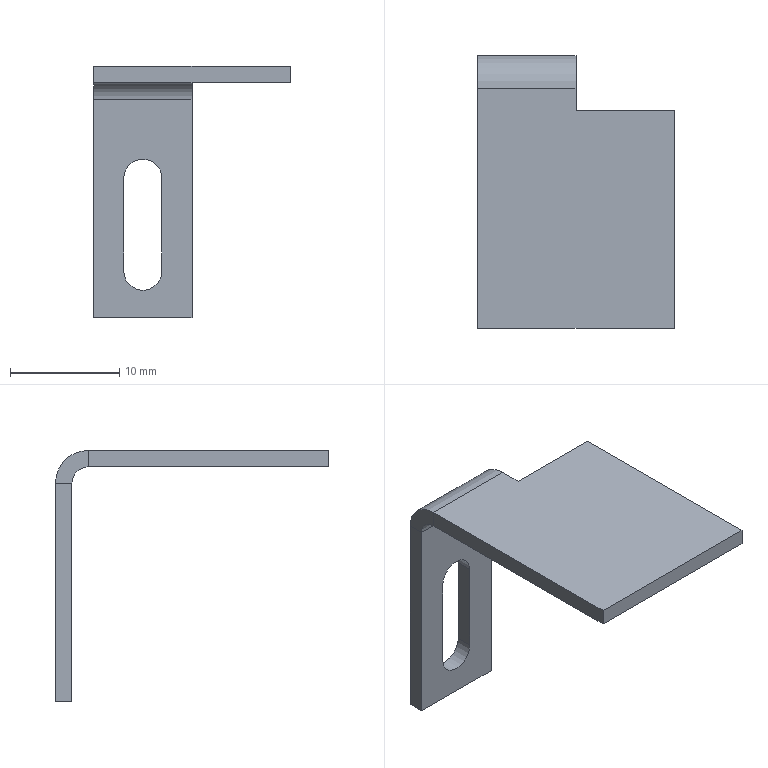Part | STEP file | Cup gripper drive lower limit bracket 1001 | 1 solid | 21 faces | box 18 x 25 x 23 mm | volume 825.656 mm3 | plane 16 | cylinder 5 | commonest cylinder face diameters 3.5 x3 3 x1 6 x1
STEP:
#1=CARTESIAN_POINT('',(0.,0.,0.));
#2=DIRECTION('',(0.,0.,1.));
#3=DIRECTION('',(1.,0.,0.));
#4=AXIS2_PLACEMENT_3D('',#1,#2,#3);
#5=CARTESIAN_POINT('',(-2.75,-1.5,1.25));
#6=VERTEX_POINT('',#5);
#7=CARTESIAN_POINT('',(-2.75,0.,1.25));
#8=VERTEX_POINT('',#7);
#9=CARTESIAN_POINT('',(-2.75,-3.,1.25));
#10=DIRECTION('',(0.,1.,0.));
#11=VECTOR('',#10,1.);
#12=LINE('',#9,#11);
#13=CARTESIAN_POINT('',(-4.5,-3.,1.25));
#14=DIRECTION('',(0.,1.,0.));
#15=DIRECTION('',(0.,0.,1.));
#16=AXIS2_PLACEMENT_3D('',#13,#14,#15);
#17=CYLINDRICAL_SURFACE('',#16,1.75);
#18=CARTESIAN_POINT('',(1.571,0.));
#19=DIRECTION('',(0.,1.));
#20=VECTOR('',#19,1.);
#21=LINE('',#18,#20);
#22=(GEOMETRIC_REPRESENTATION_CONTEXT(2)PARAMETRIC_REPRESENTATION_CONTEXT()REPRESENTATION_CONTEXT('',''));
#23=DEFINITIONAL_REPRESENTATION('',(#21),#22);
#24=PCURVE('',#17,#23);
#25=CARTESIAN_POINT('',(-2.75,-3.,1.25));
#26=DIRECTION('',(1.,0.,0.));
#27=DIRECTION('',(0.,0.,-1.));
#28=AXIS2_PLACEMENT_3D('',#25,#26,#27);
#29=PLANE('',#28);
#30=CARTESIAN_POINT('',(0.,0.));
#31=DIRECTION('',(0.,1.));
#32=VECTOR('',#31,1.);
#33=LINE('',#30,#32);
#34=(GEOMETRIC_REPRESENTATION_CONTEXT(2)PARAMETRIC_REPRESENTATION_CONTEXT()REPRESENTATION_CONTEXT('',''));
#35=DEFINITIONAL_REPRESENTATION('',(#33),#34);
#36=PCURVE('',#29,#35);
#37=SURFACE_CURVE('',#12,(#24,#36),.PCURVE_S1.);
#38=EDGE_CURVE('',#6,#8,#37,.T.);
#39=ORIENTED_EDGE('',*,*,#38,.T.);
#40=CARTESIAN_POINT('',(-4.5,0.,3.));
#41=VERTEX_POINT('',#40);
#42=CARTESIAN_POINT('',(-4.5,0.,1.25));
#43=DIRECTION('',(0.,1.,0.));
#44=DIRECTION('',(0.,0.,1.));
#45=AXIS2_PLACEMENT_3D('',#42,#43,#44);
#46=CIRCLE('',#45,1.75);
#47=CARTESIAN_POINT('',(0.,3.));
#48=DIRECTION('',(1.,0.));
#49=VECTOR('',#48,1.);
#50=LINE('',#47,#49);
#51=(GEOMETRIC_REPRESENTATION_CONTEXT(2)PARAMETRIC_REPRESENTATION_CONTEXT()REPRESENTATION_CONTEXT('',''));
#52=DEFINITIONAL_REPRESENTATION('',(#50),#51);
#53=PCURVE('',#17,#52);
#54=CARTESIAN_POINT('',(0.,0.,0.));
#55=DIRECTION('',(0.,-1.,0.));
#56=DIRECTION('',(0.,0.,-1.));
#57=AXIS2_PLACEMENT_3D('',#54,#55,#56);
#58=PLANE('',#57);
#59=CARTESIAN_POINT('',(-3.,-4.5));
#60=CARTESIAN_POINT('',(-3.,-1.469));
#61=CARTESIAN_POINT('',(-0.375,-2.984));
#62=CARTESIAN_POINT('',(2.25,-4.5));
#63=CARTESIAN_POINT('',(-0.375,-6.016));
#64=CARTESIAN_POINT('',(-3.,-7.531));
#65=CARTESIAN_POINT('',(-3.,-4.5));
#66=(BOUNDED_CURVE()B_SPLINE_CURVE(2,(#59,#60,#61,#62,#63,#64,#65),.UNSPECIFIED.,.T.,.F.)B_SPLINE_CURVE_WITH_KNOTS((1,2,2,2,2,1),(-2.094,0.,2.094,4.189,6.283,8.378),.UNSPECIFIED.)CURVE()GEOMETRIC_REPRESENTATION_ITEM()RATIONAL_B_SPLINE_CURVE((1.,0.5,1.,0.5,1.,0.5,1.))REPRESENTATION_ITEM(''));
#67=(GEOMETRIC_REPRESENTATION_CONTEXT(2)PARAMETRIC_REPRESENTATION_CONTEXT()REPRESENTATION_CONTEXT('',''));
#68=DEFINITIONAL_REPRESENTATION('',(#66),#67);
#69=PCURVE('',#58,#68);
#70=SURFACE_CURVE('',#46,(#53,#69),.PCURVE_S1.);
#71=EDGE_CURVE('',#41,#8,#70,.T.);
#72=ORIENTED_EDGE('',*,*,#71,.F.);
#73=CARTESIAN_POINT('',(-4.5,-1.5,3.));
#74=VERTEX_POINT('',#73);
#75=CARTESIAN_POINT('',(-4.5,-3.,3.));
#76=DIRECTION('',(0.,1.,0.));
#77=VECTOR('',#76,1.);
#78=LINE('',#75,#77);
#79=CARTESIAN_POINT('',(0.,0.));
#80=DIRECTION('',(0.,1.));
#81=VECTOR('',#80,1.);
#82=LINE('',#79,#81);
#83=(GEOMETRIC_REPRESENTATION_CONTEXT(2)PARAMETRIC_REPRESENTATION_CONTEXT()REPRESENTATION_CONTEXT('',''));
#84=DEFINITIONAL_REPRESENTATION('',(#82),#83);
#85=PCURVE('',#17,#84);
#86=CARTESIAN_POINT('',(-4.5,-3.,1.25));
#87=DIRECTION('',(0.,1.,0.));
#88=DIRECTION('',(0.,0.,1.));
#89=AXIS2_PLACEMENT_3D('',#86,#87,#88);
#90=CYLINDRICAL_SURFACE('',#89,1.75);
#91=CARTESIAN_POINT('',(6.283,0.));
#92=DIRECTION('',(0.,1.));
#93=VECTOR('',#92,1.);
#94=LINE('',#91,#93);
#95=(GEOMETRIC_REPRESENTATION_CONTEXT(2)PARAMETRIC_REPRESENTATION_CONTEXT()REPRESENTATION_CONTEXT('',''));
#96=DEFINITIONAL_REPRESENTATION('',(#94),#95);
#97=PCURVE('',#90,#96);
#98=SURFACE_CURVE('',#78,(#85,#97),.PCURVE_S1.);
#99=EDGE_CURVE('',#74,#41,#98,.T.);
#100=ORIENTED_EDGE('',*,*,#99,.F.);
#101=CARTESIAN_POINT('',(-4.5,-1.5,1.25));
#102=DIRECTION('',(0.,-1.,0.));
#103=DIRECTION('',(0.,0.,-1.));
#104=AXIS2_PLACEMENT_3D('',#101,#102,#103);
#105=CIRCLE('',#104,1.75);
#106=CARTESIAN_POINT('',(3.142,1.5));
#107=DIRECTION('',(-1.,0.));
#108=VECTOR('',#107,1.);
#109=LINE('',#106,#108);
#110=(GEOMETRIC_REPRESENTATION_CONTEXT(2)PARAMETRIC_REPRESENTATION_CONTEXT()REPRESENTATION_CONTEXT('',''));
#111=DEFINITIONAL_REPRESENTATION('',(#109),#110);
#112=PCURVE('',#17,#111);
#113=CARTESIAN_POINT('',(0.,-1.5,0.));
#114=DIRECTION('',(0.,-1.,0.));
#115=DIRECTION('',(0.,0.,-1.));
#116=AXIS2_PLACEMENT_3D('',#113,#114,#115);
#117=PLANE('',#116);
#118=CARTESIAN_POINT('',(-1.25,-4.5));
#119=DIRECTION('',(1.,0.));
#120=AXIS2_PLACEMENT_2D('',#118,#119);
#121=CIRCLE('',#120,1.75);
#122=(GEOMETRIC_REPRESENTATION_CONTEXT(2)PARAMETRIC_REPRESENTATION_CONTEXT()REPRESENTATION_CONTEXT('',''));
#123=DEFINITIONAL_REPRESENTATION('',(#121),#122);
#124=PCURVE('',#117,#123);
#125=SURFACE_CURVE('',#105,(#112,#124),.PCURVE_S1.);
#126=EDGE_CURVE('',#6,#74,#125,.T.);
#127=ORIENTED_EDGE('',*,*,#126,.F.);
#128=EDGE_LOOP('',(#39,#72,#100,#127));
#129=FACE_BOUND('',#128,.F.);
#130=ADVANCED_FACE('',(#129),#17,.F.);
#131=CARTESIAN_POINT('',(0.,-3.,10.));
#132=VERTEX_POINT('',#131);
#133=CARTESIAN_POINT('',(0.,-5.,10.));
#134=VERTEX_POINT('',#133);
#135=CARTESIAN_POINT('',(0.,0.,10.));
#136=DIRECTION('',(0.,-1.,0.));
#137=VECTOR('',#136,1.);
#138=LINE('',#135,#137);
#139=CARTESIAN_POINT('',(0.,-5.,-11.5));
#140=DIRECTION('',(-1.,0.,0.));
#141=DIRECTION('',(0.,0.,1.));
#142=AXIS2_PLACEMENT_3D('',#139,#140,#141);
#143=PLANE('',#142);
#144=CARTESIAN_POINT('',(21.5,5.));
#145=DIRECTION('',(0.,-1.));
#146=VECTOR('',#145,1.);
#147=LINE('',#144,#146);
#148=(GEOMETRIC_REPRESENTATION_CONTEXT(2)PARAMETRIC_REPRESENTATION_CONTEXT()REPRESENTATION_CONTEXT('',''));
#149=DEFINITIONAL_REPRESENTATION('',(#147),#148);
#150=PCURVE('',#143,#149);
#151=CARTESIAN_POINT('',(0.,0.,10.));
#152=DIRECTION('',(0.,0.,1.));
#153=DIRECTION('',(0.,-1.,0.));
#154=AXIS2_PLACEMENT_3D('',#151,#152,#153);
#155=PLANE('',#154);
#156=CARTESIAN_POINT('',(0.,0.));
#157=DIRECTION('',(1.,0.));
#158=VECTOR('',#157,1.);
#159=LINE('',#156,#158);
#160=(GEOMETRIC_REPRESENTATION_CONTEXT(2)PARAMETRIC_REPRESENTATION_CONTEXT()REPRESENTATION_CONTEXT('',''));
#161=DEFINITIONAL_REPRESENTATION('',(#159),#160);
#162=PCURVE('',#155,#161);
#163=SURFACE_CURVE('',#138,(#150,#162),.PCURVE_S1.);
#164=EDGE_CURVE('',#132,#134,#163,.T.);
#165=ORIENTED_EDGE('',*,*,#164,.F.);
#166=CARTESIAN_POINT('',(0.,-3.,11.5));
#167=VERTEX_POINT('',#166);
#168=CARTESIAN_POINT('',(0.,-3.,10.));
#169=DIRECTION('',(0.,0.,1.));
#170=VECTOR('',#169,1.);
#171=LINE('',#168,#170);
#172=CARTESIAN_POINT('',(21.5,2.));
#173=DIRECTION('',(1.,0.));
#174=VECTOR('',#173,1.);
#175=LINE('',#172,#174);
#176=(GEOMETRIC_REPRESENTATION_CONTEXT(2)PARAMETRIC_REPRESENTATION_CONTEXT()REPRESENTATION_CONTEXT('',''));
#177=DEFINITIONAL_REPRESENTATION('',(#175),#176);
#178=PCURVE('',#143,#177);
#179=CARTESIAN_POINT('',(0.,-5.,-11.5));
#180=DIRECTION('',(-1.,0.,0.));
#181=DIRECTION('',(0.,0.,1.));
#182=AXIS2_PLACEMENT_3D('',#179,#180,#181);
#183=PLANE('',#182);
#184=CARTESIAN_POINT('',(21.5,2.));
#185=DIRECTION('',(1.,0.));
#186=VECTOR('',#185,1.);
#187=LINE('',#184,#186);
#188=(GEOMETRIC_REPRESENTATION_CONTEXT(2)PARAMETRIC_REPRESENTATION_CONTEXT()REPRESENTATION_CONTEXT('',''));
#189=DEFINITIONAL_REPRESENTATION('',(#187),#188);
#190=PCURVE('',#183,#189);
#191=SURFACE_CURVE('',#171,(#178,#190),.PCURVE_S1.);
#192=EDGE_CURVE('',#132,#167,#191,.T.);
#193=ORIENTED_EDGE('',*,*,#192,.T.);
#194=CARTESIAN_POINT('',(0.,-5.,11.5));
#195=VERTEX_POINT('',#194);
#196=CARTESIAN_POINT('',(0.,-5.,11.5));
#197=DIRECTION('',(0.,1.,0.));
#198=VECTOR('',#197,1.);
#199=LINE('',#196,#198);
#200=CARTESIAN_POINT('',(23.,0.));
#201=DIRECTION('',(0.,1.));
#202=VECTOR('',#201,1.);
#203=LINE('',#200,#202);
#204=(GEOMETRIC_REPRESENTATION_CONTEXT(2)PARAMETRIC_REPRESENTATION_CONTEXT()REPRESENTATION_CONTEXT('',''));
#205=DEFINITIONAL_REPRESENTATION('',(#203),#204);
#206=PCURVE('',#143,#205);
#207=CARTESIAN_POINT('',(0.,0.,11.5));
#208=DIRECTION('',(0.,0.,1.));
#209=DIRECTION('',(0.,-1.,0.));
#210=AXIS2_PLACEMENT_3D('',#207,#208,#209);
#211=PLANE('',#210);
#212=CARTESIAN_POINT('',(5.,0.));
#213=DIRECTION('',(-1.,0.));
#214=VECTOR('',#213,1.);
#215=LINE('',#212,#214);
#216=(GEOMETRIC_REPRESENTATION_CONTEXT(2)PARAMETRIC_REPRESENTATION_CONTEXT()REPRESENTATION_CONTEXT('',''));
#217=DEFINITIONAL_REPRESENTATION('',(#215),#216);
#218=PCURVE('',#211,#217);
#219=SURFACE_CURVE('',#199,(#206,#218),.PCURVE_S1.);
#220=EDGE_CURVE('',#195,#167,#219,.T.);
#221=ORIENTED_EDGE('',*,*,#220,.F.);
#222=CARTESIAN_POINT('',(0.,-5.,-11.5));
#223=DIRECTION('',(0.,0.,1.));
#224=VECTOR('',#223,1.);
#225=LINE('',#222,#224);
#226=CARTESIAN_POINT('',(0.,0.));
#227=DIRECTION('',(1.,0.));
#228=VECTOR('',#227,1.);
#229=LINE('',#226,#228);
#230=(GEOMETRIC_REPRESENTATION_CONTEXT(2)PARAMETRIC_REPRESENTATION_CONTEXT()REPRESENTATION_CONTEXT('',''));
#231=DEFINITIONAL_REPRESENTATION('',(#229),#230);
#232=PCURVE('',#143,#231);
#233=CARTESIAN_POINT('',(0.,-5.,0.));
#234=DIRECTION('',(0.,1.,0.));
#235=DIRECTION('',(0.,0.,1.));
#236=AXIS2_PLACEMENT_3D('',#233,#234,#235);
#237=PLANE('',#236);
#238=CARTESIAN_POINT('',(-11.5,0.));
#239=DIRECTION('',(1.,0.));
#240=VECTOR('',#239,1.);
#241=LINE('',#238,#240);
#242=(GEOMETRIC_REPRESENTATION_CONTEXT(2)PARAMETRIC_REPRESENTATION_CONTEXT()REPRESENTATION_CONTEXT('',''));
#243=DEFINITIONAL_REPRESENTATION('',(#241),#242);
#244=PCURVE('',#237,#243);
#245=SURFACE_CURVE('',#225,(#232,#244),.PCURVE_S1.);
#246=EDGE_CURVE('',#134,#195,#245,.T.);
#247=ORIENTED_EDGE('',*,*,#246,.F.);
#248=EDGE_LOOP('',(#165,#193,#221,#247));
#249=FACE_BOUND('',#248,.T.);
#250=ADVANCED_FACE('',(#249),#143,.F.);
#251=CARTESIAN_POINT('',(0.,0.,-11.5));
#252=VERTEX_POINT('',#251);
#253=CARTESIAN_POINT('',(0.,0.,8.5));
#254=VERTEX_POINT('',#253);
#255=CARTESIAN_POINT('',(0.,0.,-11.5));
#256=DIRECTION('',(0.,0.,1.));
#257=VECTOR('',#256,1.);
#258=LINE('',#255,#257);
#259=CARTESIAN_POINT('',(0.,-5.,-11.5));
#260=DIRECTION('',(-1.,0.,0.));
#261=DIRECTION('',(0.,0.,1.));
#262=AXIS2_PLACEMENT_3D('',#259,#260,#261);
#263=PLANE('',#262);
#264=CARTESIAN_POINT('',(0.,5.));
#265=DIRECTION('',(1.,0.));
#266=VECTOR('',#265,1.);
#267=LINE('',#264,#266);
#268=(GEOMETRIC_REPRESENTATION_CONTEXT(2)PARAMETRIC_REPRESENTATION_CONTEXT()REPRESENTATION_CONTEXT('',''));
#269=DEFINITIONAL_REPRESENTATION('',(#267),#268);
#270=PCURVE('',#263,#269);
#271=CARTESIAN_POINT('',(11.5,0.));
#272=DIRECTION('',(-1.,0.));
#273=VECTOR('',#272,1.);
#274=LINE('',#271,#273);
#275=(GEOMETRIC_REPRESENTATION_CONTEXT(2)PARAMETRIC_REPRESENTATION_CONTEXT()REPRESENTATION_CONTEXT('',''));
#276=DEFINITIONAL_REPRESENTATION('',(#274),#275);
#277=PCURVE('',#58,#276);
#278=SURFACE_CURVE('',#258,(#270,#277),.PCURVE_S1.);
#279=EDGE_CURVE('',#252,#254,#278,.T.);
#280=ORIENTED_EDGE('',*,*,#279,.T.);
#281=CARTESIAN_POINT('',(0.,-1.5,8.5));
#282=VERTEX_POINT('',#281);
#283=CARTESIAN_POINT('',(0.,0.,8.5));
#284=DIRECTION('',(0.,-1.,0.));
#285=VECTOR('',#284,1.);
#286=LINE('',#283,#285);
#287=CARTESIAN_POINT('',(20.,5.));
#288=DIRECTION('',(0.,-1.));
#289=VECTOR('',#288,1.);
#290=LINE('',#287,#289);
#291=(GEOMETRIC_REPRESENTATION_CONTEXT(2)PARAMETRIC_REPRESENTATION_CONTEXT()REPRESENTATION_CONTEXT('',''));
#292=DEFINITIONAL_REPRESENTATION('',(#290),#291);
#293=PCURVE('',#263,#292);
#294=CARTESIAN_POINT('',(20.,5.));
#295=DIRECTION('',(0.,-1.));
#296=VECTOR('',#295,1.);
#297=LINE('',#294,#296);
#298=(GEOMETRIC_REPRESENTATION_CONTEXT(2)PARAMETRIC_REPRESENTATION_CONTEXT()REPRESENTATION_CONTEXT('',''));
#299=DEFINITIONAL_REPRESENTATION('',(#297),#298);
#300=PCURVE('',#183,#299);
#301=SURFACE_CURVE('',#286,(#293,#300),.PCURVE_S1.);
#302=EDGE_CURVE('',#254,#282,#301,.T.);
#303=ORIENTED_EDGE('',*,*,#302,.T.);
#304=CARTESIAN_POINT('',(0.,-1.5,-11.5));
#305=VERTEX_POINT('',#304);
#306=CARTESIAN_POINT('',(0.,-1.5,0.));
#307=DIRECTION('',(0.,0.,-1.));
#308=VECTOR('',#307,1.);
#309=LINE('',#306,#308);
#310=CARTESIAN_POINT('',(11.5,3.5));
#311=DIRECTION('',(-1.,0.));
#312=VECTOR('',#311,1.);
#313=LINE('',#310,#312);
#314=(GEOMETRIC_REPRESENTATION_CONTEXT(2)PARAMETRIC_REPRESENTATION_CONTEXT()REPRESENTATION_CONTEXT('',''));
#315=DEFINITIONAL_REPRESENTATION('',(#313),#314);
#316=PCURVE('',#263,#315);
#317=CARTESIAN_POINT('',(0.,0.));
#318=DIRECTION('',(1.,0.));
#319=VECTOR('',#318,1.);
#320=LINE('',#317,#319);
#321=(GEOMETRIC_REPRESENTATION_CONTEXT(2)PARAMETRIC_REPRESENTATION_CONTEXT()REPRESENTATION_CONTEXT('',''));
#322=DEFINITIONAL_REPRESENTATION('',(#320),#321);
#323=PCURVE('',#117,#322);
#324=SURFACE_CURVE('',#309,(#316,#323),.PCURVE_S1.);
#325=EDGE_CURVE('',#282,#305,#324,.T.);
#326=ORIENTED_EDGE('',*,*,#325,.T.);
#327=CARTESIAN_POINT('',(0.,-5.,-11.5));
#328=DIRECTION('',(0.,1.,0.));
#329=VECTOR('',#328,1.);
#330=LINE('',#327,#329);
#331=CARTESIAN_POINT('',(0.,0.));
#332=DIRECTION('',(0.,1.));
#333=VECTOR('',#332,1.);
#334=LINE('',#331,#333);
#335=(GEOMETRIC_REPRESENTATION_CONTEXT(2)PARAMETRIC_REPRESENTATION_CONTEXT()REPRESENTATION_CONTEXT('',''));
#336=DEFINITIONAL_REPRESENTATION('',(#334),#335);
#337=PCURVE('',#263,#336);
#338=CARTESIAN_POINT('',(-9.,-1.5,-11.5));
#339=DIRECTION('',(0.,0.,-1.));
#340=DIRECTION('',(-1.,0.,0.));
#341=AXIS2_PLACEMENT_3D('',#338,#339,#340);
#342=PLANE('',#341);
#343=CARTESIAN_POINT('',(-9.,-3.5));
#344=DIRECTION('',(0.,1.));
#345=VECTOR('',#344,1.);
#346=LINE('',#343,#345);
#347=(GEOMETRIC_REPRESENTATION_CONTEXT(2)PARAMETRIC_REPRESENTATION_CONTEXT()REPRESENTATION_CONTEXT('',''));
#348=DEFINITIONAL_REPRESENTATION('',(#346),#347);
#349=PCURVE('',#342,#348);
#350=SURFACE_CURVE('',#330,(#337,#349),.PCURVE_S1.);
#351=EDGE_CURVE('',#305,#252,#350,.T.);
#352=ORIENTED_EDGE('',*,*,#351,.T.);
#353=EDGE_LOOP('',(#280,#303,#326,#352));
#354=FACE_BOUND('',#353,.T.);
#355=ADVANCED_FACE('',(#354),#263,.F.);
#356=CARTESIAN_POINT('',(9.,-5.,10.));
#357=VERTEX_POINT('',#356);
#358=CARTESIAN_POINT('',(9.,-25.,10.));
#359=VERTEX_POINT('',#358);
#360=CARTESIAN_POINT('',(9.,0.,10.));
#361=DIRECTION('',(0.,-1.,0.));
#362=VECTOR('',#361,1.);
#363=LINE('',#360,#362);
#364=CARTESIAN_POINT('',(9.,-25.,11.5));
#365=DIRECTION('',(1.,0.,0.));
#366=DIRECTION('',(0.,1.,0.));
#367=AXIS2_PLACEMENT_3D('',#364,#365,#366);
#368=PLANE('',#367);
#369=CARTESIAN_POINT('',(25.,-1.5));
#370=DIRECTION('',(-1.,0.));
#371=VECTOR('',#370,1.);
#372=LINE('',#369,#371);
#373=(GEOMETRIC_REPRESENTATION_CONTEXT(2)PARAMETRIC_REPRESENTATION_CONTEXT()REPRESENTATION_CONTEXT('',''));
#374=DEFINITIONAL_REPRESENTATION('',(#372),#373);
#375=PCURVE('',#368,#374);
#376=CARTESIAN_POINT('',(0.,9.));
#377=DIRECTION('',(1.,0.));
#378=VECTOR('',#377,1.);
#379=LINE('',#376,#378);
#380=(GEOMETRIC_REPRESENTATION_CONTEXT(2)PARAMETRIC_REPRESENTATION_CONTEXT()REPRESENTATION_CONTEXT('',''));
#381=DEFINITIONAL_REPRESENTATION('',(#379),#380);
#382=PCURVE('',#155,#381);
#383=SURFACE_CURVE('',#363,(#375,#382),.PCURVE_S1.);
#384=EDGE_CURVE('',#357,#359,#383,.T.);
#385=ORIENTED_EDGE('',*,*,#384,.F.);
#386=CARTESIAN_POINT('',(9.,-5.,11.5));
#387=VERTEX_POINT('',#386);
#388=CARTESIAN_POINT('',(9.,-5.,-11.5));
#389=DIRECTION('',(0.,0.,-1.));
#390=VECTOR('',#389,1.);
#391=LINE('',#388,#390);
#392=CARTESIAN_POINT('',(20.,-23.));
#393=DIRECTION('',(0.,-1.));
#394=VECTOR('',#393,1.);
#395=LINE('',#392,#394);
#396=(GEOMETRIC_REPRESENTATION_CONTEXT(2)PARAMETRIC_REPRESENTATION_CONTEXT()REPRESENTATION_CONTEXT('',''));
#397=DEFINITIONAL_REPRESENTATION('',(#395),#396);
#398=PCURVE('',#368,#397);
#399=CARTESIAN_POINT('',(-11.5,9.));
#400=DIRECTION('',(-1.,0.));
#401=VECTOR('',#400,1.);
#402=LINE('',#399,#401);
#403=(GEOMETRIC_REPRESENTATION_CONTEXT(2)PARAMETRIC_REPRESENTATION_CONTEXT()REPRESENTATION_CONTEXT('',''));
#404=DEFINITIONAL_REPRESENTATION('',(#402),#403);
#405=PCURVE('',#237,#404);
#406=SURFACE_CURVE('',#391,(#398,#405),.PCURVE_S1.);
#407=EDGE_CURVE('',#387,#357,#406,.T.);
#408=ORIENTED_EDGE('',*,*,#407,.F.);
#409=CARTESIAN_POINT('',(9.,-25.,11.5));
#410=VERTEX_POINT('',#409);
#411=CARTESIAN_POINT('',(9.,-25.,11.5));
#412=DIRECTION('',(0.,-1.,0.));
#413=VECTOR('',#412,1.);
#414=LINE('',#411,#413);
#415=CARTESIAN_POINT('',(0.,0.));
#416=DIRECTION('',(-1.,0.));
#417=VECTOR('',#416,1.);
#418=LINE('',#415,#417);
#419=(GEOMETRIC_REPRESENTATION_CONTEXT(2)PARAMETRIC_REPRESENTATION_CONTEXT()REPRESENTATION_CONTEXT('',''));
#420=DEFINITIONAL_REPRESENTATION('',(#418),#419);
#421=PCURVE('',#368,#420);
#422=CARTESIAN_POINT('',(25.,9.));
#423=DIRECTION('',(1.,0.));
#424=VECTOR('',#423,1.);
#425=LINE('',#422,#424);
#426=(GEOMETRIC_REPRESENTATION_CONTEXT(2)PARAMETRIC_REPRESENTATION_CONTEXT()REPRESENTATION_CONTEXT('',''));
#427=DEFINITIONAL_REPRESENTATION('',(#425),#426);
#428=PCURVE('',#211,#427);
#429=SURFACE_CURVE('',#414,(#421,#428),.PCURVE_S1.);
#430=EDGE_CURVE('',#387,#410,#429,.T.);
#431=ORIENTED_EDGE('',*,*,#430,.T.);
#432=CARTESIAN_POINT('',(9.,-25.,11.5));
#433=DIRECTION('',(0.,0.,-1.));
#434=VECTOR('',#433,1.);
#435=LINE('',#432,#434);
#436=CARTESIAN_POINT('',(0.,0.));
#437=DIRECTION('',(0.,-1.));
#438=VECTOR('',#437,1.);
#439=LINE('',#436,#438);
#440=(GEOMETRIC_REPRESENTATION_CONTEXT(2)PARAMETRIC_REPRESENTATION_CONTEXT()REPRESENTATION_CONTEXT('',''));
#441=DEFINITIONAL_REPRESENTATION('',(#439),#440);
#442=PCURVE('',#368,#441);
#443=CARTESIAN_POINT('',(-9.,-25.,11.5));
#444=DIRECTION('',(0.,-1.,0.));
#445=DIRECTION('',(0.,0.,-1.));
#446=AXIS2_PLACEMENT_3D('',#443,#444,#445);
#447=PLANE('',#446);
#448=CARTESIAN_POINT('',(0.,18.));
#449=DIRECTION('',(1.,0.));
#450=VECTOR('',#449,1.);
#451=LINE('',#448,#450);
#452=(GEOMETRIC_REPRESENTATION_CONTEXT(2)PARAMETRIC_REPRESENTATION_CONTEXT()REPRESENTATION_CONTEXT('',''));
#453=DEFINITIONAL_REPRESENTATION('',(#451),#452);
#454=PCURVE('',#447,#453);
#455=SURFACE_CURVE('',#435,(#442,#454),.PCURVE_S1.);
#456=EDGE_CURVE('',#410,#359,#455,.T.);
#457=ORIENTED_EDGE('',*,*,#456,.T.);
#458=EDGE_LOOP('',(#385,#408,#431,#457));
#459=FACE_BOUND('',#458,.T.);
#460=ADVANCED_FACE('',(#459),#368,.T.);
#461=CARTESIAN_POINT('',(-9.,-1.5,-11.5));
#462=VERTEX_POINT('',#461);
#463=CARTESIAN_POINT('',(-9.,-1.5,8.5));
#464=VERTEX_POINT('',#463);
#465=CARTESIAN_POINT('',(-9.,-1.5,11.5));
#466=DIRECTION('',(0.,0.,1.));
#467=VECTOR('',#466,1.);
#468=LINE('',#465,#467);
#469=CARTESIAN_POINT('',(-9.,-1.5,11.5));
#470=DIRECTION('',(-1.,0.,0.));
#471=DIRECTION('',(0.,0.,1.));
#472=AXIS2_PLACEMENT_3D('',#469,#470,#471);
#473=PLANE('',#472);
#474=CARTESIAN_POINT('',(0.,0.));
#475=DIRECTION('',(1.,0.));
#476=VECTOR('',#475,1.);
#477=LINE('',#474,#476);
#478=(GEOMETRIC_REPRESENTATION_CONTEXT(2)PARAMETRIC_REPRESENTATION_CONTEXT()REPRESENTATION_CONTEXT('',''));
#479=DEFINITIONAL_REPRESENTATION('',(#477),#478);
#480=PCURVE('',#473,#479);
#481=CARTESIAN_POINT('',(-11.5,-9.));
#482=DIRECTION('',(-1.,0.));
#483=VECTOR('',#482,1.);
#484=LINE('',#481,#483);
#485=(GEOMETRIC_REPRESENTATION_CONTEXT(2)PARAMETRIC_REPRESENTATION_CONTEXT()REPRESENTATION_CONTEXT('',''));
#486=DEFINITIONAL_REPRESENTATION('',(#484),#485);
#487=PCURVE('',#117,#486);
#488=SURFACE_CURVE('',#468,(#480,#487),.PCURVE_S1.);
#489=EDGE_CURVE('',#462,#464,#488,.T.);
#490=ORIENTED_EDGE('',*,*,#489,.T.);
#491=CARTESIAN_POINT('',(-9.,0.,8.5));
#492=VERTEX_POINT('',#491);
#493=CARTESIAN_POINT('',(-9.,-1.5,8.5));
#494=DIRECTION('',(0.,1.,0.));
#495=VECTOR('',#494,1.);
#496=LINE('',#493,#495);
#497=CARTESIAN_POINT('',(-3.,0.));
#498=DIRECTION('',(0.,1.));
#499=VECTOR('',#498,1.);
#500=LINE('',#497,#499);
#501=(GEOMETRIC_REPRESENTATION_CONTEXT(2)PARAMETRIC_REPRESENTATION_CONTEXT()REPRESENTATION_CONTEXT('',''));
#502=DEFINITIONAL_REPRESENTATION('',(#500),#501);
#503=PCURVE('',#473,#502);
#504=CARTESIAN_POINT('',(-9.,-3.,8.5));
#505=DIRECTION('',(1.,0.,0.));
#506=DIRECTION('',(0.,0.,-1.));
#507=AXIS2_PLACEMENT_3D('',#504,#505,#506);
#508=PLANE('',#507);
#509=CARTESIAN_POINT('',(0.,1.5));
#510=DIRECTION('',(0.,1.));
#511=VECTOR('',#510,1.);
#512=LINE('',#509,#511);
#513=(GEOMETRIC_REPRESENTATION_CONTEXT(2)PARAMETRIC_REPRESENTATION_CONTEXT()REPRESENTATION_CONTEXT('',''));
#514=DEFINITIONAL_REPRESENTATION('',(#512),#513);
#515=PCURVE('',#508,#514);
#516=SURFACE_CURVE('',#496,(#503,#515),.PCURVE_S1.);
#517=EDGE_CURVE('',#464,#492,#516,.T.);
#518=ORIENTED_EDGE('',*,*,#517,.T.);
#519=CARTESIAN_POINT('',(-9.,0.,-11.5));
#520=VERTEX_POINT('',#519);
#521=CARTESIAN_POINT('',(-9.,0.,11.5));
#522=DIRECTION('',(0.,0.,1.));
#523=VECTOR('',#522,1.);
#524=LINE('',#521,#523);
#525=CARTESIAN_POINT('',(0.,1.5));
#526=DIRECTION('',(1.,0.));
#527=VECTOR('',#526,1.);
#528=LINE('',#525,#527);
#529=(GEOMETRIC_REPRESENTATION_CONTEXT(2)PARAMETRIC_REPRESENTATION_CONTEXT()REPRESENTATION_CONTEXT('',''));
#530=DEFINITIONAL_REPRESENTATION('',(#528),#529);
#531=PCURVE('',#473,#530);
#532=CARTESIAN_POINT('',(-11.5,-9.));
#533=DIRECTION('',(-1.,0.));
#534=VECTOR('',#533,1.);
#535=LINE('',#532,#534);
#536=(GEOMETRIC_REPRESENTATION_CONTEXT(2)PARAMETRIC_REPRESENTATION_CONTEXT()REPRESENTATION_CONTEXT('',''));
#537=DEFINITIONAL_REPRESENTATION('',(#535),#536);
#538=PCURVE('',#58,#537);
#539=SURFACE_CURVE('',#524,(#531,#538),.PCURVE_S1.);
#540=EDGE_CURVE('',#520,#492,#539,.T.);
#541=ORIENTED_EDGE('',*,*,#540,.F.);
#542=CARTESIAN_POINT('',(-9.,-1.5,-11.5));
#543=DIRECTION('',(0.,1.,0.));
#544=VECTOR('',#543,1.);
#545=LINE('',#542,#544);
#546=CARTESIAN_POINT('',(-23.,0.));
#547=DIRECTION('',(0.,1.));
#548=VECTOR('',#547,1.);
#549=LINE('',#546,#548);
#550=(GEOMETRIC_REPRESENTATION_CONTEXT(2)PARAMETRIC_REPRESENTATION_CONTEXT()REPRESENTATION_CONTEXT('',''));
#551=DEFINITIONAL_REPRESENTATION('',(#549),#550);
#552=PCURVE('',#473,#551);
#553=CARTESIAN_POINT('',(0.,0.));
#554=DIRECTION('',(0.,1.));
#555=VECTOR('',#554,1.);
#556=LINE('',#553,#555);
#557=(GEOMETRIC_REPRESENTATION_CONTEXT(2)PARAMETRIC_REPRESENTATION_CONTEXT()REPRESENTATION_CONTEXT('',''));
#558=DEFINITIONAL_REPRESENTATION('',(#556),#557);
#559=PCURVE('',#342,#558);
#560=SURFACE_CURVE('',#545,(#552,#559),.PCURVE_S1.);
#561=EDGE_CURVE('',#462,#520,#560,.T.);
#562=ORIENTED_EDGE('',*,*,#561,.F.);
#563=EDGE_LOOP('',(#490,#518,#541,#562));
#564=FACE_BOUND('',#563,.T.);
#565=ADVANCED_FACE('',(#564),#473,.T.);
#566=ORIENTED_EDGE('',*,*,#126,.F.);
#567=CARTESIAN_POINT('',(-2.75,-1.5,-7.25));
#568=VERTEX_POINT('',#567);
#569=CARTESIAN_POINT('',(-2.75,-1.5,0.));
#570=DIRECTION('',(0.,0.,1.));
#571=VECTOR('',#570,1.);
#572=LINE('',#569,#571);
#573=CARTESIAN_POINT('',(0.,-2.75));
#574=DIRECTION('',(-1.,0.));
#575=VECTOR('',#574,1.);
#576=LINE('',#573,#575);
#577=(GEOMETRIC_REPRESENTATION_CONTEXT(2)PARAMETRIC_REPRESENTATION_CONTEXT()REPRESENTATION_CONTEXT('',''));
#578=DEFINITIONAL_REPRESENTATION('',(#576),#577);
#579=PCURVE('',#117,#578);
#580=CARTESIAN_POINT('',(1.25,1.5));
#581=DIRECTION('',(-1.,0.));
#582=VECTOR('',#581,1.);
#583=LINE('',#580,#582);
#584=(GEOMETRIC_REPRESENTATION_CONTEXT(2)PARAMETRIC_REPRESENTATION_CONTEXT()REPRESENTATION_CONTEXT('',''));
#585=DEFINITIONAL_REPRESENTATION('',(#583),#584);
#586=PCURVE('',#29,#585);
#587=SURFACE_CURVE('',#572,(#579,#586),.PCURVE_S1.);
#588=EDGE_CURVE('',#568,#6,#587,.T.);
#589=ORIENTED_EDGE('',*,*,#588,.F.);
#590=CARTESIAN_POINT('',(-6.25,-1.5,-7.25));
#591=VERTEX_POINT('',#590);
#592=CARTESIAN_POINT('',(-4.5,-1.5,-7.25));
#593=DIRECTION('',(0.,-1.,0.));
#594=DIRECTION('',(0.,0.,-1.));
#595=AXIS2_PLACEMENT_3D('',#592,#593,#594);
#596=CIRCLE('',#595,1.75);
#597=CARTESIAN_POINT('',(7.25,-4.5));
#598=DIRECTION('',(1.,0.));
#599=AXIS2_PLACEMENT_2D('',#597,#598);
#600=CIRCLE('',#599,1.75);
#601=(GEOMETRIC_REPRESENTATION_CONTEXT(2)PARAMETRIC_REPRESENTATION_CONTEXT()REPRESENTATION_CONTEXT('',''));
#602=DEFINITIONAL_REPRESENTATION('',(#600),#601);
#603=PCURVE('',#117,#602);
#604=CARTESIAN_POINT('',(-4.5,-3.,-7.25));
#605=DIRECTION('',(0.,1.,0.));
#606=DIRECTION('',(0.,0.,1.));
#607=AXIS2_PLACEMENT_3D('',#604,#605,#606);
#608=CYLINDRICAL_SURFACE('',#607,1.75);
#609=CARTESIAN_POINT('',(9.425,1.5));
#610=DIRECTION('',(-1.,0.));
#611=VECTOR('',#610,1.);
#612=LINE('',#609,#611);
#613=(GEOMETRIC_REPRESENTATION_CONTEXT(2)PARAMETRIC_REPRESENTATION_CONTEXT()REPRESENTATION_CONTEXT('',''));
#614=DEFINITIONAL_REPRESENTATION('',(#612),#613);
#615=PCURVE('',#608,#614);
#616=SURFACE_CURVE('',#596,(#603,#615),.PCURVE_S1.);
#617=EDGE_CURVE('',#591,#568,#616,.T.);
#618=ORIENTED_EDGE('',*,*,#617,.F.);
#619=CARTESIAN_POINT('',(-6.25,-1.5,1.25));
#620=VERTEX_POINT('',#619);
#621=CARTESIAN_POINT('',(-6.25,-1.5,0.));
#622=DIRECTION('',(0.,0.,-1.));
#623=VECTOR('',#622,1.);
#624=LINE('',#621,#623);
#625=CARTESIAN_POINT('',(0.,-6.25));
#626=DIRECTION('',(1.,0.));
#627=VECTOR('',#626,1.);
#628=LINE('',#625,#627);
#629=(GEOMETRIC_REPRESENTATION_CONTEXT(2)PARAMETRIC_REPRESENTATION_CONTEXT()REPRESENTATION_CONTEXT('',''));
#630=DEFINITIONAL_REPRESENTATION('',(#628),#629);
#631=PCURVE('',#117,#630);
#632=CARTESIAN_POINT('',(-6.25,-3.,1.25));
#633=DIRECTION('',(-1.,0.,0.));
#634=DIRECTION('',(0.,0.,1.));
#635=AXIS2_PLACEMENT_3D('',#632,#633,#634);
#636=PLANE('',#635);
#637=CARTESIAN_POINT('',(-1.25,1.5));
#638=DIRECTION('',(-1.,0.));
#639=VECTOR('',#638,1.);
#640=LINE('',#637,#639);
#641=(GEOMETRIC_REPRESENTATION_CONTEXT(2)PARAMETRIC_REPRESENTATION_CONTEXT()REPRESENTATION_CONTEXT('',''));
#642=DEFINITIONAL_REPRESENTATION('',(#640),#641);
#643=PCURVE('',#636,#642);
#644=SURFACE_CURVE('',#624,(#631,#643),.PCURVE_S1.);
#645=EDGE_CURVE('',#620,#591,#644,.T.);
#646=ORIENTED_EDGE('',*,*,#645,.F.);
#647=CARTESIAN_POINT('',(-4.5,-1.5,1.25));
#648=DIRECTION('',(0.,-1.,0.));
#649=DIRECTION('',(0.,0.,-1.));
#650=AXIS2_PLACEMENT_3D('',#647,#648,#649);
#651=CIRCLE('',#650,1.75);
#652=CARTESIAN_POINT('',(-1.25,-4.5));
#653=DIRECTION('',(1.,0.));
#654=AXIS2_PLACEMENT_2D('',#652,#653);
#655=CIRCLE('',#654,1.75);
#656=(GEOMETRIC_REPRESENTATION_CONTEXT(2)PARAMETRIC_REPRESENTATION_CONTEXT()REPRESENTATION_CONTEXT('',''));
#657=DEFINITIONAL_REPRESENTATION('',(#655),#656);
#658=PCURVE('',#117,#657);
#659=CARTESIAN_POINT('',(9.425,1.5));
#660=DIRECTION('',(-1.,0.));
#661=VECTOR('',#660,1.);
#662=LINE('',#659,#661);
#663=(GEOMETRIC_REPRESENTATION_CONTEXT(2)PARAMETRIC_REPRESENTATION_CONTEXT()REPRESENTATION_CONTEXT('',''));
#664=DEFINITIONAL_REPRESENTATION('',(#662),#663);
#665=PCURVE('',#90,#664);
#666=SURFACE_CURVE('',#651,(#658,#665),.PCURVE_S1.);
#667=EDGE_CURVE('',#74,#620,#666,.T.);
#668=ORIENTED_EDGE('',*,*,#667,.F.);
#669=EDGE_LOOP('',(#566,#589,#618,#646,#668));
#670=FACE_BOUND('',#669,.T.);
#671=ORIENTED_EDGE('',*,*,#325,.F.);
#672=CARTESIAN_POINT('',(-9.,-1.5,8.5));
#673=DIRECTION('',(1.,0.,0.));
#674=VECTOR('',#673,1.);
#675=LINE('',#672,#674);
#676=CARTESIAN_POINT('',(-8.5,-9.));
#677=DIRECTION('',(0.,1.));
#678=VECTOR('',#677,1.);
#679=LINE('',#676,#678);
#680=(GEOMETRIC_REPRESENTATION_CONTEXT(2)PARAMETRIC_REPRESENTATION_CONTEXT()REPRESENTATION_CONTEXT('',''));
#681=DEFINITIONAL_REPRESENTATION('',(#679),#680);
#682=PCURVE('',#117,#681);
#683=CARTESIAN_POINT('',(-9.,-3.,8.5));
#684=DIRECTION('',(-1.,0.,0.));
#685=DIRECTION('',(0.,0.,1.));
#686=AXIS2_PLACEMENT_3D('',#683,#684,#685);
#687=CYLINDRICAL_SURFACE('',#686,1.5);
#688=CARTESIAN_POINT('',(1.571,0.));
#689=DIRECTION('',(0.,-1.));
#690=VECTOR('',#689,1.);
#691=LINE('',#688,#690);
#692=(GEOMETRIC_REPRESENTATION_CONTEXT(2)PARAMETRIC_REPRESENTATION_CONTEXT()REPRESENTATION_CONTEXT('',''));
#693=DEFINITIONAL_REPRESENTATION('',(#691),#692);
#694=PCURVE('',#687,#693);
#695=SURFACE_CURVE('',#675,(#682,#694),.PCURVE_S1.);
#696=EDGE_CURVE('',#464,#282,#695,.T.);
#697=ORIENTED_EDGE('',*,*,#696,.F.);
#698=ORIENTED_EDGE('',*,*,#489,.F.);
#699=CARTESIAN_POINT('',(-9.,-1.5,-11.5));
#700=DIRECTION('',(-1.,0.,0.));
#701=VECTOR('',#700,1.);
#702=LINE('',#699,#701);
#703=CARTESIAN_POINT('',(11.5,-9.));
#704=DIRECTION('',(0.,-1.));
#705=VECTOR('',#704,1.);
#706=LINE('',#703,#705);
#707=(GEOMETRIC_REPRESENTATION_CONTEXT(2)PARAMETRIC_REPRESENTATION_CONTEXT()REPRESENTATION_CONTEXT('',''));
#708=DEFINITIONAL_REPRESENTATION('',(#706),#707);
#709=PCURVE('',#117,#708);
#710=CARTESIAN_POINT('',(0.,0.));
#711=DIRECTION('',(1.,0.));
#712=VECTOR('',#711,1.);
#713=LINE('',#710,#712);
#714=(GEOMETRIC_REPRESENTATION_CONTEXT(2)PARAMETRIC_REPRESENTATION_CONTEXT()REPRESENTATION_CONTEXT('',''));
#715=DEFINITIONAL_REPRESENTATION('',(#713),#714);
#716=PCURVE('',#342,#715);
#717=SURFACE_CURVE('',#702,(#709,#716),.PCURVE_S1.);
#718=EDGE_CURVE('',#305,#462,#717,.T.);
#719=ORIENTED_EDGE('',*,*,#718,.F.);
#720=EDGE_LOOP('',(#671,#697,#698,#719));
#721=FACE_BOUND('',#720,.T.);
#722=ADVANCED_FACE('',(#670,#721),#117,.T.);
#723=CARTESIAN_POINT('',(-2.75,0.,-7.25));
#724=VERTEX_POINT('',#723);
#725=CARTESIAN_POINT('',(-2.75,0.,1.25));
#726=DIRECTION('',(0.,0.,-1.));
#727=VECTOR('',#726,1.);
#728=LINE('',#725,#727);
#729=CARTESIAN_POINT('',(-1.25,-2.75));
#730=DIRECTION('',(1.,0.));
#731=VECTOR('',#730,1.);
#732=LINE('',#729,#731);
#733=(GEOMETRIC_REPRESENTATION_CONTEXT(2)PARAMETRIC_REPRESENTATION_CONTEXT()REPRESENTATION_CONTEXT('',''));
#734=DEFINITIONAL_REPRESENTATION('',(#732),#733);
#735=PCURVE('',#58,#734);
#736=CARTESIAN_POINT('',(0.,3.));
#737=DIRECTION('',(1.,0.));
#738=VECTOR('',#737,1.);
#739=LINE('',#736,#738);
#740=(GEOMETRIC_REPRESENTATION_CONTEXT(2)PARAMETRIC_REPRESENTATION_CONTEXT()REPRESENTATION_CONTEXT('',''));
#741=DEFINITIONAL_REPRESENTATION('',(#739),#740);
#742=PCURVE('',#29,#741);
#743=SURFACE_CURVE('',#728,(#735,#742),.PCURVE_S1.);
#744=EDGE_CURVE('',#8,#724,#743,.T.);
#745=ORIENTED_EDGE('',*,*,#744,.F.);
#746=ORIENTED_EDGE('',*,*,#71,.F.);
#747=CARTESIAN_POINT('',(-6.25,0.,1.25));
#748=VERTEX_POINT('',#747);
#749=CARTESIAN_POINT('',(-4.5,0.,1.25));
#750=DIRECTION('',(0.,1.,0.));
#751=DIRECTION('',(0.,0.,1.));
#752=AXIS2_PLACEMENT_3D('',#749,#750,#751);
#753=CIRCLE('',#752,1.75);
#754=CARTESIAN_POINT('',(-3.,-4.5));
#755=CARTESIAN_POINT('',(-3.,-1.469));
#756=CARTESIAN_POINT('',(-0.375,-2.984));
#757=CARTESIAN_POINT('',(2.25,-4.5));
#758=CARTESIAN_POINT('',(-0.375,-6.016));
#759=CARTESIAN_POINT('',(-3.,-7.531));
#760=CARTESIAN_POINT('',(-3.,-4.5));
#761=(BOUNDED_CURVE()B_SPLINE_CURVE(2,(#754,#755,#756,#757,#758,#759,#760),.UNSPECIFIED.,.T.,.F.)B_SPLINE_CURVE_WITH_KNOTS((1,2,2,2,2,1),(-2.094,0.,2.094,4.189,6.283,8.378),.UNSPECIFIED.)CURVE()GEOMETRIC_REPRESENTATION_ITEM()RATIONAL_B_SPLINE_CURVE((1.,0.5,1.,0.5,1.,0.5,1.))REPRESENTATION_ITEM(''));
#762=(GEOMETRIC_REPRESENTATION_CONTEXT(2)PARAMETRIC_REPRESENTATION_CONTEXT()REPRESENTATION_CONTEXT('',''));
#763=DEFINITIONAL_REPRESENTATION('',(#761),#762);
#764=PCURVE('',#58,#763);
#765=CARTESIAN_POINT('',(0.,3.));
#766=DIRECTION('',(1.,0.));
#767=VECTOR('',#766,1.);
#768=LINE('',#765,#767);
#769=(GEOMETRIC_REPRESENTATION_CONTEXT(2)PARAMETRIC_REPRESENTATION_CONTEXT()REPRESENTATION_CONTEXT('',''));
#770=DEFINITIONAL_REPRESENTATION('',(#768),#769);
#771=PCURVE('',#90,#770);
#772=SURFACE_CURVE('',#753,(#764,#771),.PCURVE_S1.);
#773=EDGE_CURVE('',#748,#41,#772,.T.);
#774=ORIENTED_EDGE('',*,*,#773,.F.);
#775=CARTESIAN_POINT('',(-6.25,0.,-7.25));
#776=VERTEX_POINT('',#775);
#777=CARTESIAN_POINT('',(-6.25,0.,1.25));
#778=DIRECTION('',(0.,0.,1.));
#779=VECTOR('',#778,1.);
#780=LINE('',#777,#779);
#781=CARTESIAN_POINT('',(-1.25,-6.25));
#782=DIRECTION('',(-1.,0.));
#783=VECTOR('',#782,1.);
#784=LINE('',#781,#783);
#785=(GEOMETRIC_REPRESENTATION_CONTEXT(2)PARAMETRIC_REPRESENTATION_CONTEXT()REPRESENTATION_CONTEXT('',''));
#786=DEFINITIONAL_REPRESENTATION('',(#784),#785);
#787=PCURVE('',#58,#786);
#788=CARTESIAN_POINT('',(0.,3.));
#789=DIRECTION('',(1.,0.));
#790=VECTOR('',#789,1.);
#791=LINE('',#788,#790);
#792=(GEOMETRIC_REPRESENTATION_CONTEXT(2)PARAMETRIC_REPRESENTATION_CONTEXT()REPRESENTATION_CONTEXT('',''));
#793=DEFINITIONAL_REPRESENTATION('',(#791),#792);
#794=PCURVE('',#636,#793);
#795=SURFACE_CURVE('',#780,(#787,#794),.PCURVE_S1.);
#796=EDGE_CURVE('',#776,#748,#795,.T.);
#797=ORIENTED_EDGE('',*,*,#796,.F.);
#798=CARTESIAN_POINT('',(-4.5,0.,-7.25));
#799=DIRECTION('',(0.,1.,0.));
#800=DIRECTION('',(0.,0.,1.));
#801=AXIS2_PLACEMENT_3D('',#798,#799,#800);
#802=CIRCLE('',#801,1.75);
#803=CARTESIAN_POINT('',(5.5,-4.5));
#804=CARTESIAN_POINT('',(5.5,-1.469));
#805=CARTESIAN_POINT('',(8.125,-2.984));
#806=CARTESIAN_POINT('',(10.75,-4.5));
#807=CARTESIAN_POINT('',(8.125,-6.016));
#808=CARTESIAN_POINT('',(5.5,-7.531));
#809=CARTESIAN_POINT('',(5.5,-4.5));
#810=(BOUNDED_CURVE()B_SPLINE_CURVE(2,(#803,#804,#805,#806,#807,#808,#809),.UNSPECIFIED.,.T.,.F.)B_SPLINE_CURVE_WITH_KNOTS((1,2,2,2,2,1),(-2.094,0.,2.094,4.189,6.283,8.378),.UNSPECIFIED.)CURVE()GEOMETRIC_REPRESENTATION_ITEM()RATIONAL_B_SPLINE_CURVE((1.,0.5,1.,0.5,1.,0.5,1.))REPRESENTATION_ITEM(''));
#811=(GEOMETRIC_REPRESENTATION_CONTEXT(2)PARAMETRIC_REPRESENTATION_CONTEXT()REPRESENTATION_CONTEXT('',''));
#812=DEFINITIONAL_REPRESENTATION('',(#810),#811);
#813=PCURVE('',#58,#812);
#814=CARTESIAN_POINT('',(0.,3.));
#815=DIRECTION('',(1.,0.));
#816=VECTOR('',#815,1.);
#817=LINE('',#814,#816);
#818=(GEOMETRIC_REPRESENTATION_CONTEXT(2)PARAMETRIC_REPRESENTATION_CONTEXT()REPRESENTATION_CONTEXT('',''));
#819=DEFINITIONAL_REPRESENTATION('',(#817),#818);
#820=PCURVE('',#608,#819);
#821=SURFACE_CURVE('',#802,(#813,#820),.PCURVE_S1.);
#822=EDGE_CURVE('',#724,#776,#821,.T.);
#823=ORIENTED_EDGE('',*,*,#822,.F.);
#824=EDGE_LOOP('',(#745,#746,#774,#797,#823));
#825=FACE_BOUND('',#824,.T.);
#826=CARTESIAN_POINT('',(-9.,0.,8.5));
#827=DIRECTION('',(1.,0.,0.));
#828=VECTOR('',#827,1.);
#829=LINE('',#826,#828);
#830=CARTESIAN_POINT('',(-8.5,-9.));
#831=DIRECTION('',(0.,1.));
#832=VECTOR('',#831,1.);
#833=LINE('',#830,#832);
#834=(GEOMETRIC_REPRESENTATION_CONTEXT(2)PARAMETRIC_REPRESENTATION_CONTEXT()REPRESENTATION_CONTEXT('',''));
#835=DEFINITIONAL_REPRESENTATION('',(#833),#834);
#836=PCURVE('',#58,#835);
#837=CARTESIAN_POINT('',(-9.,-3.,8.5));
#838=DIRECTION('',(-1.,0.,0.));
#839=DIRECTION('',(0.,0.,1.));
#840=AXIS2_PLACEMENT_3D('',#837,#838,#839);
#841=CYLINDRICAL_SURFACE('',#840,3.);
#842=CARTESIAN_POINT('',(1.571,0.));
#843=DIRECTION('',(0.,-1.));
#844=VECTOR('',#843,1.);
#845=LINE('',#842,#844);
#846=(GEOMETRIC_REPRESENTATION_CONTEXT(2)PARAMETRIC_REPRESENTATION_CONTEXT()REPRESENTATION_CONTEXT('',''));
#847=DEFINITIONAL_REPRESENTATION('',(#845),#846);
#848=PCURVE('',#841,#847);
#849=SURFACE_CURVE('',#829,(#836,#848),.PCURVE_S1.);
#850=EDGE_CURVE('',#492,#254,#849,.T.);
#851=ORIENTED_EDGE('',*,*,#850,.T.);
#852=ORIENTED_EDGE('',*,*,#279,.F.);
#853=CARTESIAN_POINT('',(-9.,0.,-11.5));
#854=DIRECTION('',(-1.,0.,0.));
#855=VECTOR('',#854,1.);
#856=LINE('',#853,#855);
#857=CARTESIAN_POINT('',(11.5,-9.));
#858=DIRECTION('',(0.,-1.));
#859=VECTOR('',#858,1.);
#860=LINE('',#857,#859);
#861=(GEOMETRIC_REPRESENTATION_CONTEXT(2)PARAMETRIC_REPRESENTATION_CONTEXT()REPRESENTATION_CONTEXT('',''));
#862=DEFINITIONAL_REPRESENTATION('',(#860),#861);
#863=PCURVE('',#58,#862);
#864=CARTESIAN_POINT('',(0.,1.5));
#865=DIRECTION('',(1.,0.));
#866=VECTOR('',#865,1.);
#867=LINE('',#864,#866);
#868=(GEOMETRIC_REPRESENTATION_CONTEXT(2)PARAMETRIC_REPRESENTATION_CONTEXT()REPRESENTATION_CONTEXT('',''));
#869=DEFINITIONAL_REPRESENTATION('',(#867),#868);
#870=PCURVE('',#342,#869);
#871=SURFACE_CURVE('',#856,(#863,#870),.PCURVE_S1.);
#872=EDGE_CURVE('',#252,#520,#871,.T.);
#873=ORIENTED_EDGE('',*,*,#872,.T.);
#874=ORIENTED_EDGE('',*,*,#540,.T.);
#875=EDGE_LOOP('',(#851,#852,#873,#874));
#876=FACE_BOUND('',#875,.T.);
#877=ADVANCED_FACE('',(#825,#876),#58,.F.);
#878=ORIENTED_EDGE('',*,*,#351,.F.);
#879=ORIENTED_EDGE('',*,*,#718,.T.);
#880=ORIENTED_EDGE('',*,*,#561,.T.);
#881=ORIENTED_EDGE('',*,*,#872,.F.);
#882=EDGE_LOOP('',(#878,#879,#880,#881));
#883=FACE_BOUND('',#882,.T.);
#884=ADVANCED_FACE('',(#883),#342,.T.);
#885=CARTESIAN_POINT('',(-9.,-3.,10.));
#886=VERTEX_POINT('',#885);
#887=CARTESIAN_POINT('',(-9.,-3.,8.5));
#888=DIRECTION('',(-1.,0.,0.));
#889=DIRECTION('',(0.,0.,1.));
#890=AXIS2_PLACEMENT_3D('',#887,#888,#889);
#891=CIRCLE('',#890,1.5);
#892=CARTESIAN_POINT('',(-1.5,0.));
#893=CARTESIAN_POINT('',(-1.5,2.598));
#894=CARTESIAN_POINT('',(0.75,1.299));
#895=CARTESIAN_POINT('',(3.,0.));
#896=CARTESIAN_POINT('',(0.75,-1.299));
#897=CARTESIAN_POINT('',(-1.5,-2.598));
#898=CARTESIAN_POINT('',(-1.5,0.));
#899=(BOUNDED_CURVE()B_SPLINE_CURVE(2,(#892,#893,#894,#895,#896,#897,#898),.UNSPECIFIED.,.T.,.F.)B_SPLINE_CURVE_WITH_KNOTS((1,2,2,2,2,1),(-2.094,0.,2.094,4.189,6.283,8.378),.UNSPECIFIED.)CURVE()GEOMETRIC_REPRESENTATION_ITEM()RATIONAL_B_SPLINE_CURVE((1.,0.5,1.,0.5,1.,0.5,1.))REPRESENTATION_ITEM(''));
#900=(GEOMETRIC_REPRESENTATION_CONTEXT(2)PARAMETRIC_REPRESENTATION_CONTEXT()REPRESENTATION_CONTEXT('',''));
#901=DEFINITIONAL_REPRESENTATION('',(#899),#900);
#902=PCURVE('',#508,#901);
#903=CARTESIAN_POINT('',(0.,0.));
#904=DIRECTION('',(1.,0.));
#905=VECTOR('',#904,1.);
#906=LINE('',#903,#905);
#907=(GEOMETRIC_REPRESENTATION_CONTEXT(2)PARAMETRIC_REPRESENTATION_CONTEXT()REPRESENTATION_CONTEXT('',''));
#908=DEFINITIONAL_REPRESENTATION('',(#906),#907);
#909=PCURVE('',#687,#908);
#910=SURFACE_CURVE('',#891,(#902,#909),.PCURVE_S1.);
#911=EDGE_CURVE('',#886,#464,#910,.T.);
#912=ORIENTED_EDGE('',*,*,#911,.F.);
#913=CARTESIAN_POINT('',(-9.,-3.,11.5));
#914=VERTEX_POINT('',#913);
#915=CARTESIAN_POINT('',(-9.,-3.,10.));
#916=DIRECTION('',(0.,0.,1.));
#917=VECTOR('',#916,1.);
#918=LINE('',#915,#917);
#919=CARTESIAN_POINT('',(-1.5,0.));
#920=DIRECTION('',(-1.,0.));
#921=VECTOR('',#920,1.);
#922=LINE('',#919,#921);
#923=(GEOMETRIC_REPRESENTATION_CONTEXT(2)PARAMETRIC_REPRESENTATION_CONTEXT()REPRESENTATION_CONTEXT('',''));
#924=DEFINITIONAL_REPRESENTATION('',(#922),#923);
#925=PCURVE('',#508,#924);
#926=CARTESIAN_POINT('',(-9.,-1.5,11.5));
#927=DIRECTION('',(-1.,0.,0.));
#928=DIRECTION('',(0.,-1.,0.));
#929=AXIS2_PLACEMENT_3D('',#926,#927,#928);
#930=PLANE('',#929);
#931=CARTESIAN_POINT('',(1.5,-1.5));
#932=DIRECTION('',(0.,1.));
#933=VECTOR('',#932,1.);
#934=LINE('',#931,#933);
#935=(GEOMETRIC_REPRESENTATION_CONTEXT(2)PARAMETRIC_REPRESENTATION_CONTEXT()REPRESENTATION_CONTEXT('',''));
#936=DEFINITIONAL_REPRESENTATION('',(#934),#935);
#937=PCURVE('',#930,#936);
#938=SURFACE_CURVE('',#918,(#925,#937),.PCURVE_S1.);
#939=EDGE_CURVE('',#886,#914,#938,.T.);
#940=ORIENTED_EDGE('',*,*,#939,.T.);
#941=CARTESIAN_POINT('',(-9.,-3.,8.5));
#942=DIRECTION('',(-1.,0.,0.));
#943=DIRECTION('',(0.,0.,1.));
#944=AXIS2_PLACEMENT_3D('',#941,#942,#943);
#945=CIRCLE('',#944,3.);
#946=CARTESIAN_POINT('',(-3.,0.));
#947=CARTESIAN_POINT('',(-3.,5.196));
#948=CARTESIAN_POINT('',(1.5,2.598));
#949=CARTESIAN_POINT('',(6.,0.));
#950=CARTESIAN_POINT('',(1.5,-2.598));
#951=CARTESIAN_POINT('',(-3.,-5.196));
#952=CARTESIAN_POINT('',(-3.,0.));
#953=(BOUNDED_CURVE()B_SPLINE_CURVE(2,(#946,#947,#948,#949,#950,#951,#952),.UNSPECIFIED.,.T.,.F.)B_SPLINE_CURVE_WITH_KNOTS((1,2,2,2,2,1),(-2.094,0.,2.094,4.189,6.283,8.378),.UNSPECIFIED.)CURVE()GEOMETRIC_REPRESENTATION_ITEM()RATIONAL_B_SPLINE_CURVE((1.,0.5,1.,0.5,1.,0.5,1.))REPRESENTATION_ITEM(''));
#954=(GEOMETRIC_REPRESENTATION_CONTEXT(2)PARAMETRIC_REPRESENTATION_CONTEXT()REPRESENTATION_CONTEXT('',''));
#955=DEFINITIONAL_REPRESENTATION('',(#953),#954);
#956=PCURVE('',#508,#955);
#957=CARTESIAN_POINT('',(0.,0.));
#958=DIRECTION('',(1.,0.));
#959=VECTOR('',#958,1.);
#960=LINE('',#957,#959);
#961=(GEOMETRIC_REPRESENTATION_CONTEXT(2)PARAMETRIC_REPRESENTATION_CONTEXT()REPRESENTATION_CONTEXT('',''));
#962=DEFINITIONAL_REPRESENTATION('',(#960),#961);
#963=PCURVE('',#841,#962);
#964=SURFACE_CURVE('',#945,(#956,#963),.PCURVE_S1.);
#965=EDGE_CURVE('',#914,#492,#964,.T.);
#966=ORIENTED_EDGE('',*,*,#965,.T.);
#967=ORIENTED_EDGE('',*,*,#517,.F.);
#968=EDGE_LOOP('',(#912,#940,#966,#967));
#969=FACE_BOUND('',#968,.T.);
#970=ADVANCED_FACE('',(#969),#508,.F.);
#971=CARTESIAN_POINT('',(0.,-3.,8.5));
#972=DIRECTION('',(1.,0.,0.));
#973=DIRECTION('',(0.,0.,1.));
#974=AXIS2_PLACEMENT_3D('',#971,#972,#973);
#975=CIRCLE('',#974,3.);
#976=CARTESIAN_POINT('',(6.283,-9.));
#977=DIRECTION('',(-1.,0.));
#978=VECTOR('',#977,1.);
#979=LINE('',#976,#978);
#980=(GEOMETRIC_REPRESENTATION_CONTEXT(2)PARAMETRIC_REPRESENTATION_CONTEXT()REPRESENTATION_CONTEXT('',''));
#981=DEFINITIONAL_REPRESENTATION('',(#979),#980);
#982=PCURVE('',#841,#981);
#983=CARTESIAN_POINT('',(23.,2.));
#984=CARTESIAN_POINT('',(23.,-3.196));
#985=CARTESIAN_POINT('',(18.5,-0.5981));
#986=CARTESIAN_POINT('',(14.,2.));
#987=CARTESIAN_POINT('',(18.5,4.598));
#988=CARTESIAN_POINT('',(23.,7.196));
#989=CARTESIAN_POINT('',(23.,2.));
#990=(BOUNDED_CURVE()B_SPLINE_CURVE(2,(#983,#984,#985,#986,#987,#988,#989),.UNSPECIFIED.,.T.,.F.)B_SPLINE_CURVE_WITH_KNOTS((1,2,2,2,2,1),(-2.094,0.,2.094,4.189,6.283,8.378),.UNSPECIFIED.)CURVE()GEOMETRIC_REPRESENTATION_ITEM()RATIONAL_B_SPLINE_CURVE((1.,0.5,1.,0.5,1.,0.5,1.))REPRESENTATION_ITEM(''));
#991=(GEOMETRIC_REPRESENTATION_CONTEXT(2)PARAMETRIC_REPRESENTATION_CONTEXT()REPRESENTATION_CONTEXT('',''));
#992=DEFINITIONAL_REPRESENTATION('',(#990),#991);
#993=PCURVE('',#183,#992);
#994=SURFACE_CURVE('',#975,(#982,#993),.PCURVE_S1.);
#995=EDGE_CURVE('',#254,#167,#994,.T.);
#996=ORIENTED_EDGE('',*,*,#995,.F.);
#997=ORIENTED_EDGE('',*,*,#850,.F.);
#998=ORIENTED_EDGE('',*,*,#965,.F.);
#999=CARTESIAN_POINT('',(0.,-3.,11.5));
#1000=DIRECTION('',(-1.,0.,0.));
#1001=VECTOR('',#1000,1.);
#1002=LINE('',#999,#1001);
#1003=CARTESIAN_POINT('',(0.,-9.));
#1004=DIRECTION('',(0.,1.));
#1005=VECTOR('',#1004,1.);
#1006=LINE('',#1003,#1005);
#1007=(GEOMETRIC_REPRESENTATION_CONTEXT(2)PARAMETRIC_REPRESENTATION_CONTEXT()REPRESENTATION_CONTEXT('',''));
#1008=DEFINITIONAL_REPRESENTATION('',(#1006),#1007);
#1009=PCURVE('',#841,#1008);
#1010=CARTESIAN_POINT('',(3.,0.));
#1011=DIRECTION('',(0.,-1.));
#1012=VECTOR('',#1011,1.);
#1013=LINE('',#1010,#1012);
#1014=(GEOMETRIC_REPRESENTATION_CONTEXT(2)PARAMETRIC_REPRESENTATION_CONTEXT()REPRESENTATION_CONTEXT('',''));
#1015=DEFINITIONAL_REPRESENTATION('',(#1013),#1014);
#1016=PCURVE('',#211,#1015);
#1017=SURFACE_CURVE('',#1002,(#1009,#1016),.PCURVE_S1.);
#1018=EDGE_CURVE('',#167,#914,#1017,.T.);
#1019=ORIENTED_EDGE('',*,*,#1018,.F.);
#1020=EDGE_LOOP('',(#996,#997,#998,#1019));
#1021=FACE_BOUND('',#1020,.T.);
#1022=ADVANCED_FACE('',(#1021),#841,.T.);
#1023=ORIENTED_EDGE('',*,*,#911,.F.);
#1024=CARTESIAN_POINT('',(9.,-3.,10.));
#1025=DIRECTION('',(-1.,0.,0.));
#1026=VECTOR('',#1025,1.);
#1027=LINE('',#1024,#1026);
#1028=CARTESIAN_POINT('',(0.,-18.));
#1029=DIRECTION('',(0.,1.));
#1030=VECTOR('',#1029,1.);
#1031=LINE('',#1028,#1030);
#1032=(GEOMETRIC_REPRESENTATION_CONTEXT(2)PARAMETRIC_REPRESENTATION_CONTEXT()REPRESENTATION_CONTEXT('',''));
#1033=DEFINITIONAL_REPRESENTATION('',(#1031),#1032);
#1034=PCURVE('',#687,#1033);
#1035=CARTESIAN_POINT('',(3.,9.));
#1036=DIRECTION('',(0.,-1.));
#1037=VECTOR('',#1036,1.);
#1038=LINE('',#1035,#1037);
#1039=(GEOMETRIC_REPRESENTATION_CONTEXT(2)PARAMETRIC_REPRESENTATION_CONTEXT()REPRESENTATION_CONTEXT('',''));
#1040=DEFINITIONAL_REPRESENTATION('',(#1038),#1039);
#1041=PCURVE('',#155,#1040);
#1042=SURFACE_CURVE('',#1027,(#1034,#1041),.PCURVE_S1.);
#1043=EDGE_CURVE('',#132,#886,#1042,.T.);
#1044=ORIENTED_EDGE('',*,*,#1043,.F.);
#1045=CARTESIAN_POINT('',(0.,-3.,8.5));
#1046=DIRECTION('',(1.,0.,0.));
#1047=DIRECTION('',(0.,0.,1.));
#1048=AXIS2_PLACEMENT_3D('',#1045,#1046,#1047);
#1049=CIRCLE('',#1048,1.5);
#1050=CARTESIAN_POINT('',(6.283,-9.));
#1051=DIRECTION('',(-1.,0.));
#1052=VECTOR('',#1051,1.);
#1053=LINE('',#1050,#1052);
#1054=(GEOMETRIC_REPRESENTATION_CONTEXT(2)PARAMETRIC_REPRESENTATION_CONTEXT()REPRESENTATION_CONTEXT('',''));
#1055=DEFINITIONAL_REPRESENTATION('',(#1053),#1054);
#1056=PCURVE('',#687,#1055);
#1057=CARTESIAN_POINT('',(21.5,2.));
#1058=CARTESIAN_POINT('',(21.5,-0.5981));
#1059=CARTESIAN_POINT('',(19.25,0.701));
#1060=CARTESIAN_POINT('',(17.,2.));
#1061=CARTESIAN_POINT('',(19.25,3.299));
#1062=CARTESIAN_POINT('',(21.5,4.598));
#1063=CARTESIAN_POINT('',(21.5,2.));
#1064=(BOUNDED_CURVE()B_SPLINE_CURVE(2,(#1057,#1058,#1059,#1060,#1061,#1062,#1063),.UNSPECIFIED.,.T.,.F.)B_SPLINE_CURVE_WITH_KNOTS((1,2,2,2,2,1),(-2.094,0.,2.094,4.189,6.283,8.378),.UNSPECIFIED.)CURVE()GEOMETRIC_REPRESENTATION_ITEM()RATIONAL_B_SPLINE_CURVE((1.,0.5,1.,0.5,1.,0.5,1.))REPRESENTATION_ITEM(''));
#1065=(GEOMETRIC_REPRESENTATION_CONTEXT(2)PARAMETRIC_REPRESENTATION_CONTEXT()REPRESENTATION_CONTEXT('',''));
#1066=DEFINITIONAL_REPRESENTATION('',(#1064),#1065);
#1067=PCURVE('',#183,#1066);
#1068=SURFACE_CURVE('',#1049,(#1056,#1067),.PCURVE_S1.);
#1069=EDGE_CURVE('',#282,#132,#1068,.T.);
#1070=ORIENTED_EDGE('',*,*,#1069,.F.);
#1071=ORIENTED_EDGE('',*,*,#696,.F.);
#1072=EDGE_LOOP('',(#1023,#1044,#1070,#1071));
#1073=FACE_BOUND('',#1072,.F.);
#1074=ADVANCED_FACE('',(#1073),#687,.F.);
#1075=CARTESIAN_POINT('',(-9.,-25.,11.5));
#1076=VERTEX_POINT('',#1075);
#1077=CARTESIAN_POINT('',(-9.,-1.5,11.5));
#1078=DIRECTION('',(0.,1.,0.));
#1079=VECTOR('',#1078,1.);
#1080=LINE('',#1077,#1079);
#1081=CARTESIAN_POINT('',(0.,0.));
#1082=DIRECTION('',(-1.,0.));
#1083=VECTOR('',#1082,1.);
#1084=LINE('',#1081,#1083);
#1085=(GEOMETRIC_REPRESENTATION_CONTEXT(2)PARAMETRIC_REPRESENTATION_CONTEXT()REPRESENTATION_CONTEXT('',''));
#1086=DEFINITIONAL_REPRESENTATION('',(#1084),#1085);
#1087=PCURVE('',#930,#1086);
#1088=CARTESIAN_POINT('',(1.5,-9.));
#1089=DIRECTION('',(-1.,0.));
#1090=VECTOR('',#1089,1.);
#1091=LINE('',#1088,#1090);
#1092=(GEOMETRIC_REPRESENTATION_CONTEXT(2)PARAMETRIC_REPRESENTATION_CONTEXT()REPRESENTATION_CONTEXT('',''));
#1093=DEFINITIONAL_REPRESENTATION('',(#1091),#1092);
#1094=PCURVE('',#211,#1093);
#1095=SURFACE_CURVE('',#1080,(#1087,#1094),.PCURVE_S1.);
#1096=EDGE_CURVE('',#1076,#914,#1095,.T.);
#1097=ORIENTED_EDGE('',*,*,#1096,.T.);
#1098=ORIENTED_EDGE('',*,*,#939,.F.);
#1099=CARTESIAN_POINT('',(-9.,-25.,10.));
#1100=VERTEX_POINT('',#1099);
#1101=CARTESIAN_POINT('',(-9.,0.,10.));
#1102=DIRECTION('',(0.,1.,0.));
#1103=VECTOR('',#1102,1.);
#1104=LINE('',#1101,#1103);
#1105=CARTESIAN_POINT('',(-1.5,-1.5));
#1106=DIRECTION('',(-1.,0.));
#1107=VECTOR('',#1106,1.);
#1108=LINE('',#1105,#1107);
#1109=(GEOMETRIC_REPRESENTATION_CONTEXT(2)PARAMETRIC_REPRESENTATION_CONTEXT()REPRESENTATION_CONTEXT('',''));
#1110=DEFINITIONAL_REPRESENTATION('',(#1108),#1109);
#1111=PCURVE('',#930,#1110);
#1112=CARTESIAN_POINT('',(0.,-9.));
#1113=DIRECTION('',(-1.,0.));
#1114=VECTOR('',#1113,1.);
#1115=LINE('',#1112,#1114);
#1116=(GEOMETRIC_REPRESENTATION_CONTEXT(2)PARAMETRIC_REPRESENTATION_CONTEXT()REPRESENTATION_CONTEXT('',''));
#1117=DEFINITIONAL_REPRESENTATION('',(#1115),#1116);
#1118=PCURVE('',#155,#1117);
#1119=SURFACE_CURVE('',#1104,(#1111,#1118),.PCURVE_S1.);
#1120=EDGE_CURVE('',#1100,#886,#1119,.T.);
#1121=ORIENTED_EDGE('',*,*,#1120,.F.);
#1122=CARTESIAN_POINT('',(-9.,-25.,11.5));
#1123=DIRECTION('',(0.,0.,-1.));
#1124=VECTOR('',#1123,1.);
#1125=LINE('',#1122,#1124);
#1126=CARTESIAN_POINT('',(23.5,0.));
#1127=DIRECTION('',(0.,-1.));
#1128=VECTOR('',#1127,1.);
#1129=LINE('',#1126,#1128);
#1130=(GEOMETRIC_REPRESENTATION_CONTEXT(2)PARAMETRIC_REPRESENTATION_CONTEXT()REPRESENTATION_CONTEXT('',''));
#1131=DEFINITIONAL_REPRESENTATION('',(#1129),#1130);
#1132=PCURVE('',#930,#1131);
#1133=CARTESIAN_POINT('',(0.,0.));
#1134=DIRECTION('',(1.,0.));
#1135=VECTOR('',#1134,1.);
#1136=LINE('',#1133,#1135);
#1137=(GEOMETRIC_REPRESENTATION_CONTEXT(2)PARAMETRIC_REPRESENTATION_CONTEXT()REPRESENTATION_CONTEXT('',''));
#1138=DEFINITIONAL_REPRESENTATION('',(#1136),#1137);
#1139=PCURVE('',#447,#1138);
#1140=SURFACE_CURVE('',#1125,(#1132,#1139),.PCURVE_S1.);
#1141=EDGE_CURVE('',#1076,#1100,#1140,.T.);
#1142=ORIENTED_EDGE('',*,*,#1141,.F.);
#1143=EDGE_LOOP('',(#1097,#1098,#1121,#1142));
#1144=FACE_BOUND('',#1143,.T.);
#1145=ADVANCED_FACE('',(#1144),#930,.T.);
#1146=ORIENTED_EDGE('',*,*,#220,.T.);
#1147=ORIENTED_EDGE('',*,*,#1018,.T.);
#1148=ORIENTED_EDGE('',*,*,#1096,.F.);
#1149=CARTESIAN_POINT('',(-9.,-25.,11.5));
#1150=DIRECTION('',(-1.,0.,0.));
#1151=VECTOR('',#1150,1.);
#1152=LINE('',#1149,#1151);
#1153=CARTESIAN_POINT('',(25.,-9.));
#1154=DIRECTION('',(0.,-1.));
#1155=VECTOR('',#1154,1.);
#1156=LINE('',#1153,#1155);
#1157=(GEOMETRIC_REPRESENTATION_CONTEXT(2)PARAMETRIC_REPRESENTATION_CONTEXT()REPRESENTATION_CONTEXT('',''));
#1158=DEFINITIONAL_REPRESENTATION('',(#1156),#1157);
#1159=PCURVE('',#211,#1158);
#1160=CARTESIAN_POINT('',(0.,0.));
#1161=DIRECTION('',(0.,-1.));
#1162=VECTOR('',#1161,1.);
#1163=LINE('',#1160,#1162);
#1164=(GEOMETRIC_REPRESENTATION_CONTEXT(2)PARAMETRIC_REPRESENTATION_CONTEXT()REPRESENTATION_CONTEXT('',''));
#1165=DEFINITIONAL_REPRESENTATION('',(#1163),#1164);
#1166=PCURVE('',#447,#1165);
#1167=SURFACE_CURVE('',#1152,(#1159,#1166),.PCURVE_S1.);
#1168=EDGE_CURVE('',#410,#1076,#1167,.T.);
#1169=ORIENTED_EDGE('',*,*,#1168,.F.);
#1170=ORIENTED_EDGE('',*,*,#430,.F.);
#1171=CARTESIAN_POINT('',(0.,-5.,11.5));
#1172=DIRECTION('',(1.,0.,0.));
#1173=VECTOR('',#1172,1.);
#1174=LINE('',#1171,#1173);
#1175=CARTESIAN_POINT('',(5.,0.));
#1176=DIRECTION('',(0.,1.));
#1177=VECTOR('',#1176,1.);
#1178=LINE('',#1175,#1177);
#1179=(GEOMETRIC_REPRESENTATION_CONTEXT(2)PARAMETRIC_REPRESENTATION_CONTEXT()REPRESENTATION_CONTEXT('',''));
#1180=DEFINITIONAL_REPRESENTATION('',(#1178),#1179);
#1181=PCURVE('',#211,#1180);
#1182=CARTESIAN_POINT('',(11.5,0.));
#1183=DIRECTION('',(0.,1.));
#1184=VECTOR('',#1183,1.);
#1185=LINE('',#1182,#1184);
#1186=(GEOMETRIC_REPRESENTATION_CONTEXT(2)PARAMETRIC_REPRESENTATION_CONTEXT()REPRESENTATION_CONTEXT('',''));
#1187=DEFINITIONAL_REPRESENTATION('',(#1185),#1186);
#1188=PCURVE('',#237,#1187);
#1189=SURFACE_CURVE('',#1174,(#1181,#1188),.PCURVE_S1.);
#1190=EDGE_CURVE('',#195,#387,#1189,.T.);
#1191=ORIENTED_EDGE('',*,*,#1190,.F.);
#1192=EDGE_LOOP('',(#1146,#1147,#1148,#1169,#1170,#1191));
#1193=FACE_BOUND('',#1192,.T.);
#1194=ADVANCED_FACE('',(#1193),#211,.T.);
#1195=ORIENTED_EDGE('',*,*,#1043,.F.);
#1196=ORIENTED_EDGE('',*,*,#164,.T.);
#1197=CARTESIAN_POINT('',(0.,-5.,10.));
#1198=DIRECTION('',(-1.,0.,0.));
#1199=VECTOR('',#1198,1.);
#1200=LINE('',#1197,#1199);
#1201=CARTESIAN_POINT('',(5.,0.));
#1202=DIRECTION('',(0.,-1.));
#1203=VECTOR('',#1202,1.);
#1204=LINE('',#1201,#1203);
#1205=(GEOMETRIC_REPRESENTATION_CONTEXT(2)PARAMETRIC_REPRESENTATION_CONTEXT()REPRESENTATION_CONTEXT('',''));
#1206=DEFINITIONAL_REPRESENTATION('',(#1204),#1205);
#1207=PCURVE('',#155,#1206);
#1208=CARTESIAN_POINT('',(10.,0.));
#1209=DIRECTION('',(0.,-1.));
#1210=VECTOR('',#1209,1.);
#1211=LINE('',#1208,#1210);
#1212=(GEOMETRIC_REPRESENTATION_CONTEXT(2)PARAMETRIC_REPRESENTATION_CONTEXT()REPRESENTATION_CONTEXT('',''));
#1213=DEFINITIONAL_REPRESENTATION('',(#1211),#1212);
#1214=PCURVE('',#237,#1213);
#1215=SURFACE_CURVE('',#1200,(#1207,#1214),.PCURVE_S1.);
#1216=EDGE_CURVE('',#357,#134,#1215,.T.);
#1217=ORIENTED_EDGE('',*,*,#1216,.F.);
#1218=ORIENTED_EDGE('',*,*,#384,.T.);
#1219=CARTESIAN_POINT('',(0.,-25.,10.));
#1220=DIRECTION('',(-1.,0.,0.));
#1221=VECTOR('',#1220,1.);
#1222=LINE('',#1219,#1221);
#1223=CARTESIAN_POINT('',(25.,0.));
#1224=DIRECTION('',(0.,-1.));
#1225=VECTOR('',#1224,1.);
#1226=LINE('',#1223,#1225);
#1227=(GEOMETRIC_REPRESENTATION_CONTEXT(2)PARAMETRIC_REPRESENTATION_CONTEXT()REPRESENTATION_CONTEXT('',''));
#1228=DEFINITIONAL_REPRESENTATION('',(#1226),#1227);
#1229=PCURVE('',#155,#1228);
#1230=CARTESIAN_POINT('',(1.5,9.));
#1231=DIRECTION('',(0.,-1.));
#1232=VECTOR('',#1231,1.);
#1233=LINE('',#1230,#1232);
#1234=(GEOMETRIC_REPRESENTATION_CONTEXT(2)PARAMETRIC_REPRESENTATION_CONTEXT()REPRESENTATION_CONTEXT('',''));
#1235=DEFINITIONAL_REPRESENTATION('',(#1233),#1234);
#1236=PCURVE('',#447,#1235);
#1237=SURFACE_CURVE('',#1222,(#1229,#1236),.PCURVE_S1.);
#1238=EDGE_CURVE('',#359,#1100,#1237,.T.);
#1239=ORIENTED_EDGE('',*,*,#1238,.T.);
#1240=ORIENTED_EDGE('',*,*,#1120,.T.);
#1241=EDGE_LOOP('',(#1195,#1196,#1217,#1218,#1239,#1240));
#1242=FACE_BOUND('',#1241,.T.);
#1243=ADVANCED_FACE('',(#1242),#155,.F.);
#1244=ORIENTED_EDGE('',*,*,#1238,.F.);
#1245=ORIENTED_EDGE('',*,*,#456,.F.);
#1246=ORIENTED_EDGE('',*,*,#1168,.T.);
#1247=ORIENTED_EDGE('',*,*,#1141,.T.);
#1248=EDGE_LOOP('',(#1244,#1245,#1246,#1247));
#1249=FACE_BOUND('',#1248,.T.);
#1250=ADVANCED_FACE('',(#1249),#447,.T.);
#1251=ORIENTED_EDGE('',*,*,#1216,.T.);
#1252=ORIENTED_EDGE('',*,*,#246,.T.);
#1253=ORIENTED_EDGE('',*,*,#1190,.T.);
#1254=ORIENTED_EDGE('',*,*,#407,.T.);
#1255=EDGE_LOOP('',(#1251,#1252,#1253,#1254));
#1256=FACE_BOUND('',#1255,.T.);
#1257=ADVANCED_FACE('',(#1256),#237,.T.);
#1258=ORIENTED_EDGE('',*,*,#192,.F.);
#1259=ORIENTED_EDGE('',*,*,#1069,.F.);
#1260=ORIENTED_EDGE('',*,*,#302,.F.);
#1261=ORIENTED_EDGE('',*,*,#995,.T.);
#1262=EDGE_LOOP('',(#1258,#1259,#1260,#1261));
#1263=FACE_BOUND('',#1262,.T.);
#1264=ADVANCED_FACE('',(#1263),#183,.F.);
#1265=ORIENTED_EDGE('',*,*,#773,.F.);
#1266=CARTESIAN_POINT('',(-6.25,-3.,1.25));
#1267=DIRECTION('',(0.,1.,0.));
#1268=VECTOR('',#1267,1.);
#1269=LINE('',#1266,#1268);
#1270=CARTESIAN_POINT('',(4.712,0.));
#1271=DIRECTION('',(0.,1.));
#1272=VECTOR('',#1271,1.);
#1273=LINE('',#1270,#1272);
#1274=(GEOMETRIC_REPRESENTATION_CONTEXT(2)PARAMETRIC_REPRESENTATION_CONTEXT()REPRESENTATION_CONTEXT('',''));
#1275=DEFINITIONAL_REPRESENTATION('',(#1273),#1274);
#1276=PCURVE('',#90,#1275);
#1277=CARTESIAN_POINT('',(0.,0.));
#1278=DIRECTION('',(0.,1.));
#1279=VECTOR('',#1278,1.);
#1280=LINE('',#1277,#1279);
#1281=(GEOMETRIC_REPRESENTATION_CONTEXT(2)PARAMETRIC_REPRESENTATION_CONTEXT()REPRESENTATION_CONTEXT('',''));
#1282=DEFINITIONAL_REPRESENTATION('',(#1280),#1281);
#1283=PCURVE('',#636,#1282);
#1284=SURFACE_CURVE('',#1269,(#1276,#1283),.PCURVE_S1.);
#1285=EDGE_CURVE('',#620,#748,#1284,.T.);
#1286=ORIENTED_EDGE('',*,*,#1285,.F.);
#1287=ORIENTED_EDGE('',*,*,#667,.F.);
#1288=ORIENTED_EDGE('',*,*,#99,.T.);
#1289=EDGE_LOOP('',(#1265,#1286,#1287,#1288));
#1290=FACE_BOUND('',#1289,.F.);
#1291=ADVANCED_FACE('',(#1290),#90,.F.);
#1292=ORIENTED_EDGE('',*,*,#645,.T.);
#1293=CARTESIAN_POINT('',(-6.25,-3.,-7.25));
#1294=DIRECTION('',(0.,1.,0.));
#1295=VECTOR('',#1294,1.);
#1296=LINE('',#1293,#1295);
#1297=CARTESIAN_POINT('',(-8.5,0.));
#1298=DIRECTION('',(0.,1.));
#1299=VECTOR('',#1298,1.);
#1300=LINE('',#1297,#1299);
#1301=(GEOMETRIC_REPRESENTATION_CONTEXT(2)PARAMETRIC_REPRESENTATION_CONTEXT()REPRESENTATION_CONTEXT('',''));
#1302=DEFINITIONAL_REPRESENTATION('',(#1300),#1301);
#1303=PCURVE('',#636,#1302);
#1304=CARTESIAN_POINT('',(4.712,0.));
#1305=DIRECTION('',(0.,1.));
#1306=VECTOR('',#1305,1.);
#1307=LINE('',#1304,#1306);
#1308=(GEOMETRIC_REPRESENTATION_CONTEXT(2)PARAMETRIC_REPRESENTATION_CONTEXT()REPRESENTATION_CONTEXT('',''));
#1309=DEFINITIONAL_REPRESENTATION('',(#1307),#1308);
#1310=PCURVE('',#608,#1309);
#1311=SURFACE_CURVE('',#1296,(#1303,#1310),.PCURVE_S1.);
#1312=EDGE_CURVE('',#591,#776,#1311,.T.);
#1313=ORIENTED_EDGE('',*,*,#1312,.T.);
#1314=ORIENTED_EDGE('',*,*,#796,.T.);
#1315=ORIENTED_EDGE('',*,*,#1285,.F.);
#1316=EDGE_LOOP('',(#1292,#1313,#1314,#1315));
#1317=FACE_BOUND('',#1316,.T.);
#1318=ADVANCED_FACE('',(#1317),#636,.F.);
#1319=ORIENTED_EDGE('',*,*,#1312,.T.);
#1320=ORIENTED_EDGE('',*,*,#822,.F.);
#1321=CARTESIAN_POINT('',(-2.75,-3.,-7.25));
#1322=DIRECTION('',(0.,1.,0.));
#1323=VECTOR('',#1322,1.);
#1324=LINE('',#1321,#1323);
#1325=CARTESIAN_POINT('',(1.571,0.));
#1326=DIRECTION('',(0.,1.));
#1327=VECTOR('',#1326,1.);
#1328=LINE('',#1325,#1327);
#1329=(GEOMETRIC_REPRESENTATION_CONTEXT(2)PARAMETRIC_REPRESENTATION_CONTEXT()REPRESENTATION_CONTEXT('',''));
#1330=DEFINITIONAL_REPRESENTATION('',(#1328),#1329);
#1331=PCURVE('',#608,#1330);
#1332=CARTESIAN_POINT('',(8.5,0.));
#1333=DIRECTION('',(0.,1.));
#1334=VECTOR('',#1333,1.);
#1335=LINE('',#1332,#1334);
#1336=(GEOMETRIC_REPRESENTATION_CONTEXT(2)PARAMETRIC_REPRESENTATION_CONTEXT()REPRESENTATION_CONTEXT('',''));
#1337=DEFINITIONAL_REPRESENTATION('',(#1335),#1336);
#1338=PCURVE('',#29,#1337);
#1339=SURFACE_CURVE('',#1324,(#1331,#1338),.PCURVE_S1.);
#1340=EDGE_CURVE('',#568,#724,#1339,.T.);
#1341=ORIENTED_EDGE('',*,*,#1340,.F.);
#1342=ORIENTED_EDGE('',*,*,#617,.F.);
#1343=EDGE_LOOP('',(#1319,#1320,#1341,#1342));
#1344=FACE_BOUND('',#1343,.F.);
#1345=ADVANCED_FACE('',(#1344),#608,.F.);
#1346=ORIENTED_EDGE('',*,*,#588,.T.);
#1347=ORIENTED_EDGE('',*,*,#38,.T.);
#1348=ORIENTED_EDGE('',*,*,#744,.T.);
#1349=ORIENTED_EDGE('',*,*,#1340,.F.);
#1350=EDGE_LOOP('',(#1346,#1347,#1348,#1349));
#1351=FACE_BOUND('',#1350,.T.);
#1352=ADVANCED_FACE('',(#1351),#29,.F.);
#1353=CLOSED_SHELL('',(#130,#250,#355,#460,#565,#722,#877,#884,#970,#1022,#1074,#1145,#1194,#1243,#1250,#1257,#1264,#1291,#1318,#1345,#1352));
#1354=MANIFOLD_SOLID_BREP('',#1353);
#1355=(LENGTH_UNIT()NAMED_UNIT(*)SI_UNIT(.MILLI.,.METRE.));
#1356=UNCERTAINTY_MEASURE_WITH_UNIT(LENGTH_MEASURE(0.0000001),#1355,'','');
#1357=(NAMED_UNIT(*)PLANE_ANGLE_UNIT()SI_UNIT($,.RADIAN.));
#1358=(NAMED_UNIT(*)SI_UNIT($,.STERADIAN.)SOLID_ANGLE_UNIT());
#1359=(GEOMETRIC_REPRESENTATION_CONTEXT(3)GLOBAL_UNCERTAINTY_ASSIGNED_CONTEXT((#1356))GLOBAL_UNIT_ASSIGNED_CONTEXT((#1355,#1357,#1358))REPRESENTATION_CONTEXT('',''));
#1360=ADVANCED_BREP_SHAPE_REPRESENTATION('',(#4,#1354),#1359);